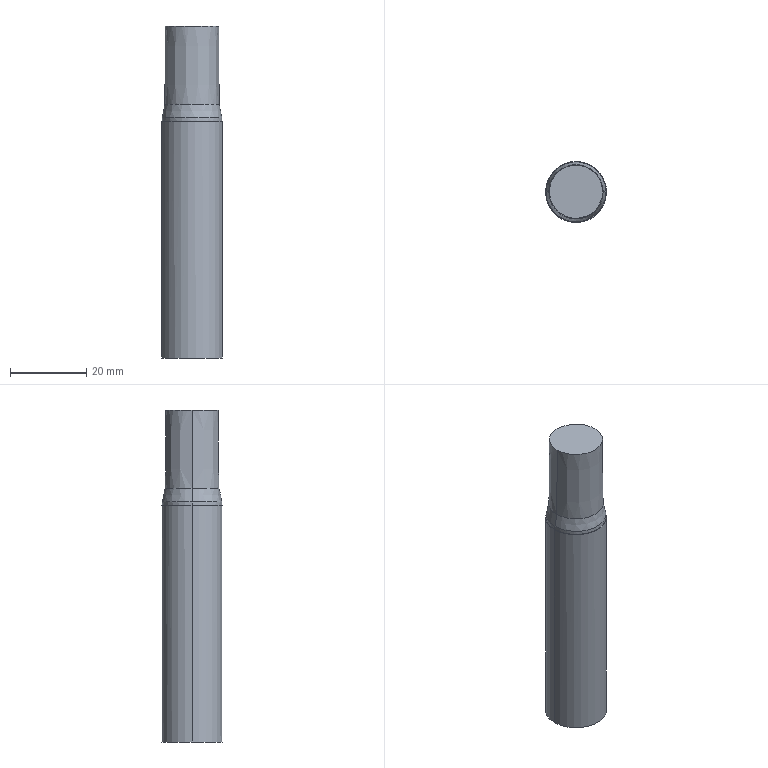Part | Creo | 1 solid | 11 faces | box 16 x 16 x 87.289 mm | volume 16530 mm3 | cylinder 4 | cone 4 | plane 3 | commonest cylinder face diameters 15.678 x2 16 x2
STEP:
#1=CARTESIAN_POINT('',(0.,0.,0.));
#2=DIRECTION('',(0.,0.,1.));
#3=DIRECTION('',(1.,0.,0.));
#4=AXIS2_PLACEMENT_3D('',#1,#2,#3);
#5=CARTESIAN_POINT('',(-166.942,-31.148,-153.441));
#6=VERTEX_POINT('',#5);
#7=CARTESIAN_POINT('',(-150.942,-31.148,-153.441));
#8=VERTEX_POINT('',#7);
#9=CARTESIAN_POINT('',(-158.942,-31.148,-153.441));
#10=DIRECTION('',(0.,0.,-1.));
#11=DIRECTION('',(-1.,0.,0.));
#12=AXIS2_PLACEMENT_3D('',#9,#10,#11);
#13=CIRCLE('',#12,8.);
#14=EDGE_CURVE('',#6,#8,#13,.T.);
#15=ORIENTED_EDGE('',*,*,#14,.T.);
#16=CARTESIAN_POINT('',(-150.942,-31.148,-91.317));
#17=VERTEX_POINT('',#16);
#18=CARTESIAN_POINT('',(-150.942,-31.148,-91.317));
#19=DIRECTION('',(0.,0.,-1.));
#20=VECTOR('',#19,62.125);
#21=LINE('',#18,#20);
#22=EDGE_CURVE('',#17,#8,#21,.T.);
#23=ORIENTED_EDGE('',*,*,#22,.F.);
#24=CARTESIAN_POINT('',(-166.942,-31.138,-91.296));
#25=VERTEX_POINT('',#24);
#26=CARTESIAN_POINT('',(-166.941,-30.196,-91.296));
#27=CARTESIAN_POINT('',(-166.597,-28.159,-91.296));
#28=CARTESIAN_POINT('',(-165.067,-25.793,-91.298));
#29=CARTESIAN_POINT('',(-163.339,-24.398,-91.301));
#30=CARTESIAN_POINT('',(-161.89,-23.654,-91.303));
#31=CARTESIAN_POINT('',(-160.637,-23.302,-91.304));
#32=CARTESIAN_POINT('',(-159.651,-23.169,-91.306));
#33=CARTESIAN_POINT('',(-158.937,-23.138,-91.306));
#34=CARTESIAN_POINT('',(-158.222,-23.17,-91.307));
#35=CARTESIAN_POINT('',(-157.236,-23.304,-91.309));
#36=CARTESIAN_POINT('',(-155.984,-23.658,-91.31));
#37=CARTESIAN_POINT('',(-154.536,-24.404,-91.312));
#38=CARTESIAN_POINT('',(-152.809,-25.801,-91.314));
#39=CARTESIAN_POINT('',(-151.283,-28.169,-91.316));
#40=CARTESIAN_POINT('',(-150.942,-30.206,-91.317));
#41=B_SPLINE_CURVE_WITH_KNOTS('',3,(#24,#26,#27,#28,#29,#30,#31,#32,#33,#34,#35,#36,#37,#38,#39,#40,#16),.UNSPECIFIED.,.F.,.F.,(4,1,1,1,1,1,1,1,1,1,1,1,1,1,4),(0.,0.125,0.25,0.3125,0.375,0.4375,0.4688,0.5,0.5312,0.5625,0.625,0.6875,0.75,0.875,1.),.UNSPECIFIED.);
#42=EDGE_CURVE('',#25,#17,#41,.T.);
#43=ORIENTED_EDGE('',*,*,#42,.F.);
#44=CARTESIAN_POINT('',(-166.942,-31.148,-91.296));
#45=VERTEX_POINT('',#44);
#46=CARTESIAN_POINT('',(-166.942,-31.145,-91.296));
#47=CARTESIAN_POINT('',(-166.942,-31.141,-91.296));
#48=CARTESIAN_POINT('',(-166.942,-31.138,-91.296));
#49=B_SPLINE_CURVE_WITH_KNOTS('',3,(#44,#46,#47,#48),.UNSPECIFIED.,.F.,.F.,(4,4),(0.,1.),.UNSPECIFIED.);
#50=EDGE_CURVE('',#45,#25,#49,.T.);
#51=ORIENTED_EDGE('',*,*,#50,.F.);
#52=CARTESIAN_POINT('',(-166.942,-31.148,-91.296));
#53=DIRECTION('',(-0.000000074,0.,-1.));
#54=VECTOR('',#53,62.146);
#55=LINE('',#52,#54);
#56=EDGE_CURVE('',#45,#6,#55,.T.);
#57=ORIENTED_EDGE('',*,*,#56,.T.);
#58=EDGE_LOOP('',(#15,#23,#43,#51,#57));
#59=FACE_OUTER_BOUND('',#58,.F.);
#60=CARTESIAN_POINT('',(-158.942,-31.148,508.193));
#61=DIRECTION('',(0.,0.,-1.));
#62=DIRECTION('',(-1.,0.,0.));
#63=AXIS2_PLACEMENT_3D('',#60,#61,#62);
#64=CYLINDRICAL_SURFACE('',#63,8.);
#65=ADVANCED_FACE('',(#59),#64,.T.);
#66=ORIENTED_EDGE('',*,*,#14,.F.);
#67=CARTESIAN_POINT('',(-158.942,-31.148,-153.441));
#68=DIRECTION('',(0.,0.,-1.));
#69=DIRECTION('',(1.,0.,0.));
#70=AXIS2_PLACEMENT_3D('',#67,#68,#69);
#71=CIRCLE('',#70,8.);
#72=EDGE_CURVE('',#8,#6,#71,.T.);
#73=ORIENTED_EDGE('',*,*,#72,.F.);
#74=EDGE_LOOP('',(#66,#73));
#75=FACE_OUTER_BOUND('',#74,.F.);
#76=CARTESIAN_POINT('',(5.725,319.968,-153.441));
#77=DIRECTION('',(0.,0.,-1.));
#78=DIRECTION('',(-1.,0.,0.));
#79=AXIS2_PLACEMENT_3D('',#76,#77,#78);
#80=PLANE('',#79);
#81=ADVANCED_FACE('',(#75),#80,.T.);
#82=ORIENTED_EDGE('',*,*,#72,.T.);
#83=ORIENTED_EDGE('',*,*,#56,.F.);
#84=CARTESIAN_POINT('',(-150.942,-31.158,-91.317));
#85=VERTEX_POINT('',#84);
#86=CARTESIAN_POINT('',(-150.942,-31.654,-91.317));
#87=CARTESIAN_POINT('',(-151.034,-32.628,-91.317));
#88=CARTESIAN_POINT('',(-151.44,-34.058,-91.316));
#89=CARTESIAN_POINT('',(-152.105,-35.389,-91.315));
#90=CARTESIAN_POINT('',(-152.991,-36.563,-91.314));
#91=CARTESIAN_POINT('',(-154.092,-37.569,-91.313));
#92=CARTESIAN_POINT('',(-155.36,-38.353,-91.311));
#93=CARTESIAN_POINT('',(-156.748,-38.889,-91.309));
#94=CARTESIAN_POINT('',(-158.208,-39.16,-91.307));
#95=CARTESIAN_POINT('',(-159.691,-39.159,-91.305));
#96=CARTESIAN_POINT('',(-161.146,-38.886,-91.304));
#97=CARTESIAN_POINT('',(-162.527,-38.35,-91.302));
#98=CARTESIAN_POINT('',(-163.788,-37.571,-91.3));
#99=CARTESIAN_POINT('',(-164.887,-36.569,-91.299));
#100=CARTESIAN_POINT('',(-165.774,-35.396,-91.297));
#101=CARTESIAN_POINT('',(-166.442,-34.063,-91.297));
#102=CARTESIAN_POINT('',(-166.85,-32.626,-91.296));
#103=CARTESIAN_POINT('',(-166.942,-31.647,-91.296));
#104=CARTESIAN_POINT('',(-166.942,-31.148,-91.296));
#105=B_SPLINE_CURVE_WITH_KNOTS('',3,(#84,#86,#87,#88,#89,#90,#91,#92,#93,#94,#95,#96,#97,#98,#99,#100,#101,#102,#103,#104),.UNSPECIFIED.,.F.,.F.,(4,1,1,1,1,1,1,1,1,1,1,1,1,1,1,1,1,4),(0.,0.05882,0.1176,0.1765,0.2353,0.2941,0.3529,0.4118,0.4706,0.5294,0.5882,0.6471,0.7059,0.7647,0.8235,0.8824,0.9412,1.),.UNSPECIFIED.);
#106=EDGE_CURVE('',#85,#45,#105,.T.);
#107=ORIENTED_EDGE('',*,*,#106,.F.);
#108=CARTESIAN_POINT('',(-150.942,-31.148,-91.317));
#109=CARTESIAN_POINT('',(-150.942,-31.152,-91.317));
#110=CARTESIAN_POINT('',(-150.942,-31.155,-91.317));
#111=CARTESIAN_POINT('',(-150.942,-31.158,-91.317));
#112=B_SPLINE_CURVE_WITH_KNOTS('',3,(#108,#109,#110,#111),.UNSPECIFIED.,.F.,.F.,(4,4),(0.,1.),.UNSPECIFIED.);
#113=EDGE_CURVE('',#17,#85,#112,.T.);
#114=ORIENTED_EDGE('',*,*,#113,.F.);
#115=ORIENTED_EDGE('',*,*,#22,.T.);
#116=EDGE_LOOP('',(#82,#83,#107,#114,#115));
#117=FACE_OUTER_BOUND('',#116,.F.);
#118=CARTESIAN_POINT('',(-158.942,-31.148,508.193));
#119=DIRECTION('',(0.,0.,-1.));
#120=DIRECTION('',(-1.,0.,0.));
#121=AXIS2_PLACEMENT_3D('',#118,#119,#120);
#122=CYLINDRICAL_SURFACE('',#121,8.);
#123=ADVANCED_FACE('',(#117),#122,.T.);
#124=ORIENTED_EDGE('',*,*,#106,.T.);
#125=ORIENTED_EDGE('',*,*,#50,.T.);
#126=ORIENTED_EDGE('',*,*,#42,.T.);
#127=ORIENTED_EDGE('',*,*,#113,.T.);
#128=EDGE_LOOP('',(#124,#125,#126,#127));
#129=FACE_OUTER_BOUND('',#128,.F.);
#130=CARTESIAN_POINT('',(-151.103,-31.158,-91.317));
#131=VERTEX_POINT('',#130);
#132=CARTESIAN_POINT('',(-151.103,-31.148,-91.317));
#133=VERTEX_POINT('',#132);
#134=CARTESIAN_POINT('',(-151.103,-31.155,-91.317));
#135=CARTESIAN_POINT('',(-151.103,-31.152,-91.317));
#136=CARTESIAN_POINT('',(-151.103,-31.148,-91.317));
#137=B_SPLINE_CURVE_WITH_KNOTS('',3,(#130,#134,#135,#136),.UNSPECIFIED.,.F.,.F.,(4,4),(0.,1.),.UNSPECIFIED.);
#138=EDGE_CURVE('',#131,#133,#137,.T.);
#139=ORIENTED_EDGE('',*,*,#138,.T.);
#140=CARTESIAN_POINT('',(-166.781,-31.138,-91.296));
#141=VERTEX_POINT('',#140);
#142=CARTESIAN_POINT('',(-151.103,-30.662,-91.317));
#143=CARTESIAN_POINT('',(-151.191,-29.708,-91.317));
#144=CARTESIAN_POINT('',(-151.587,-28.306,-91.316));
#145=CARTESIAN_POINT('',(-152.238,-27.001,-91.315));
#146=CARTESIAN_POINT('',(-153.104,-25.85,-91.314));
#147=CARTESIAN_POINT('',(-154.181,-24.863,-91.313));
#148=CARTESIAN_POINT('',(-155.422,-24.093,-91.311));
#149=CARTESIAN_POINT('',(-156.782,-23.566,-91.309));
#150=CARTESIAN_POINT('',(-158.213,-23.298,-91.307));
#151=CARTESIAN_POINT('',(-159.665,-23.298,-91.305));
#152=CARTESIAN_POINT('',(-161.092,-23.564,-91.304));
#153=CARTESIAN_POINT('',(-162.446,-24.086,-91.302));
#154=CARTESIAN_POINT('',(-163.683,-24.849,-91.3));
#155=CARTESIAN_POINT('',(-164.76,-25.829,-91.299));
#156=CARTESIAN_POINT('',(-165.631,-26.977,-91.298));
#157=CARTESIAN_POINT('',(-166.287,-28.283,-91.297));
#158=CARTESIAN_POINT('',(-166.689,-29.69,-91.296));
#159=CARTESIAN_POINT('',(-166.78,-30.65,-91.296));
#160=CARTESIAN_POINT('',(-166.781,-31.138,-91.296));
#161=B_SPLINE_CURVE_WITH_KNOTS('',3,(#132,#142,#143,#144,#145,#146,#147,#148,#149,#150,#151,#152,#153,#154,#155,#156,#157,#158,#159,#160),.UNSPECIFIED.,.F.,.F.,(4,1,1,1,1,1,1,1,1,1,1,1,1,1,1,1,1,4),(0.,0.05882,0.1176,0.1765,0.2353,0.2941,0.3529,0.4118,0.4706,0.5294,0.5882,0.6471,0.7059,0.7647,0.8235,0.8824,0.9412,1.),.UNSPECIFIED.);
#162=EDGE_CURVE('',#133,#141,#161,.T.);
#163=ORIENTED_EDGE('',*,*,#162,.T.);
#164=CARTESIAN_POINT('',(-166.781,-31.148,-91.296));
#165=VERTEX_POINT('',#164);
#166=CARTESIAN_POINT('',(-166.781,-31.142,-91.296));
#167=CARTESIAN_POINT('',(-166.781,-31.145,-91.296));
#168=B_SPLINE_CURVE_WITH_KNOTS('',3,(#140,#166,#167,#164),.UNSPECIFIED.,.F.,.F.,(4,4),(0.,1.),.UNSPECIFIED.);
#169=EDGE_CURVE('',#141,#165,#168,.T.);
#170=ORIENTED_EDGE('',*,*,#169,.T.);
#171=CARTESIAN_POINT('',(-166.781,-31.148,-91.296));
#172=CARTESIAN_POINT('',(-166.781,-32.072,-91.296));
#173=CARTESIAN_POINT('',(-166.446,-34.068,-91.297));
#174=CARTESIAN_POINT('',(-164.951,-36.388,-91.299));
#175=CARTESIAN_POINT('',(-163.259,-37.757,-91.301));
#176=CARTESIAN_POINT('',(-161.84,-38.488,-91.303));
#177=CARTESIAN_POINT('',(-160.613,-38.835,-91.304));
#178=CARTESIAN_POINT('',(-159.647,-38.966,-91.306));
#179=CARTESIAN_POINT('',(-158.947,-38.997,-91.306));
#180=CARTESIAN_POINT('',(-158.247,-38.967,-91.307));
#181=CARTESIAN_POINT('',(-157.28,-38.837,-91.309));
#182=CARTESIAN_POINT('',(-156.053,-38.491,-91.31));
#183=CARTESIAN_POINT('',(-154.633,-37.763,-91.312));
#184=CARTESIAN_POINT('',(-152.94,-36.395,-91.314));
#185=CARTESIAN_POINT('',(-151.441,-34.077,-91.316));
#186=CARTESIAN_POINT('',(-151.104,-32.082,-91.317));
#187=CARTESIAN_POINT('',(-151.103,-31.158,-91.317));
#188=B_SPLINE_CURVE_WITH_KNOTS('',3,(#171,#172,#173,#174,#175,#176,#177,#178,#179,#180,#181,#182,#183,#184,#185,#186,#187),.UNSPECIFIED.,.F.,.F.,(4,1,1,1,1,1,1,1,1,1,1,1,1,1,4),(0.,0.125,0.25,0.3125,0.375,0.4375,0.4688,0.5,0.5312,0.5625,0.625,0.6875,0.75,0.875,1.),.UNSPECIFIED.);
#189=EDGE_CURVE('',#165,#131,#188,.T.);
#190=ORIENTED_EDGE('',*,*,#189,.T.);
#191=EDGE_LOOP('',(#139,#163,#170,#190));
#192=FACE_BOUND('',#191,.F.);
#193=CARTESIAN_POINT('',(248.993,54.022,-91.842));
#194=DIRECTION('',(-0.001312,0.000001665,-1.));
#195=DIRECTION('',(-1.,0.,0.001312));
#196=AXIS2_PLACEMENT_3D('',#193,#194,#195);
#197=PLANE('',#196);
#198=ADVANCED_FACE('',(#129,#192),#197,.F.);
#199=CARTESIAN_POINT('',(-166.782,-31.148,-90.301));
#200=VERTEX_POINT('',#199);
#201=CARTESIAN_POINT('',(-151.102,-31.148,-90.301));
#202=VERTEX_POINT('',#201);
#203=CARTESIAN_POINT('',(-158.943,-31.148,-90.301));
#204=DIRECTION('',(0.00002709,0.,1.));
#205=DIRECTION('',(-1.,0.,0.00002709));
#206=AXIS2_PLACEMENT_3D('',#203,#204,#205);
#207=CIRCLE('',#206,7.841);
#208=EDGE_CURVE('',#200,#202,#207,.T.);
#209=ORIENTED_EDGE('',*,*,#208,.T.);
#210=CARTESIAN_POINT('',(-151.103,-31.148,-91.317));
#211=DIRECTION('',(0.0003927,0.000000008,1.));
#212=VECTOR('',#211,1.015);
#213=LINE('',#210,#212);
#214=EDGE_CURVE('',#133,#202,#213,.T.);
#215=ORIENTED_EDGE('',*,*,#214,.F.);
#216=ORIENTED_EDGE('',*,*,#138,.F.);
#217=ORIENTED_EDGE('',*,*,#189,.F.);
#218=CARTESIAN_POINT('',(-166.781,-31.148,-91.296));
#219=DIRECTION('',(-0.001462,0.,1.));
#220=VECTOR('',#219,0.995);
#221=LINE('',#218,#220);
#222=EDGE_CURVE('',#165,#200,#221,.T.);
#223=ORIENTED_EDGE('',*,*,#222,.T.);
#224=EDGE_LOOP('',(#209,#215,#216,#217,#223));
#225=FACE_OUTER_BOUND('',#224,.F.);
#226=CARTESIAN_POINT('',(-158.942,-31.148,-91.306));
#227=DIRECTION('',(0.,0.,1.));
#228=DIRECTION('',(1.,0.,0.));
#229=AXIS2_PLACEMENT_3D('',#226,#227,#228);
#230=CYLINDRICAL_SURFACE('',#229,7.839);
#231=ADVANCED_FACE('',(#225),#230,.T.);
#232=CARTESIAN_POINT('',(-166.079,-31.148,-86.784));
#233=VERTEX_POINT('',#232);
#234=CARTESIAN_POINT('',(-151.806,-31.148,-86.784));
#235=VERTEX_POINT('',#234);
#236=CARTESIAN_POINT('',(-158.942,-31.148,-86.784));
#237=DIRECTION('',(0.,0.,1.));
#238=DIRECTION('',(-1.,0.,0.));
#239=AXIS2_PLACEMENT_3D('',#236,#237,#238);
#240=CIRCLE('',#239,7.136);
#241=EDGE_CURVE('',#233,#235,#240,.T.);
#242=ORIENTED_EDGE('',*,*,#241,.T.);
#243=CARTESIAN_POINT('',(-151.806,-31.148,-86.784));
#244=DIRECTION('',(0.1961,0.,-0.9806));
#245=VECTOR('',#244,3.587);
#246=LINE('',#243,#245);
#247=EDGE_CURVE('',#235,#202,#246,.T.);
#248=ORIENTED_EDGE('',*,*,#247,.T.);
#249=ORIENTED_EDGE('',*,*,#208,.F.);
#250=CARTESIAN_POINT('',(-166.079,-31.148,-86.784));
#251=DIRECTION('',(-0.1962,0.,-0.9806));
#252=VECTOR('',#251,3.587);
#253=LINE('',#250,#252);
#254=EDGE_CURVE('',#233,#200,#253,.T.);
#255=ORIENTED_EDGE('',*,*,#254,.F.);
#256=EDGE_LOOP('',(#242,#248,#249,#255));
#257=FACE_OUTER_BOUND('',#256,.F.);
#258=CARTESIAN_POINT('',(-158.943,-31.148,-88.542));
#259=DIRECTION('',(-0.00002709,0.,-1.));
#260=DIRECTION('',(1.,0.,-0.00002709));
#261=AXIS2_PLACEMENT_3D('',#258,#259,#260);
#262=CONICAL_SURFACE('',#261,7.489,11.313);
#263=ADVANCED_FACE('',(#257),#262,.T.);
#264=ORIENTED_EDGE('',*,*,#241,.F.);
#265=CARTESIAN_POINT('',(-165.934,-31.148,-66.216));
#266=VERTEX_POINT('',#265);
#267=CARTESIAN_POINT('',(-165.934,-31.148,-66.216));
#268=DIRECTION('',(-0.007043,0.,-1.));
#269=VECTOR('',#268,20.568);
#270=LINE('',#267,#269);
#271=EDGE_CURVE('',#266,#233,#270,.T.);
#272=ORIENTED_EDGE('',*,*,#271,.F.);
#273=CARTESIAN_POINT('',(-159.821,-38.084,-66.153));
#274=VERTEX_POINT('',#273);
#275=CARTESIAN_POINT('',(-165.934,-31.148,-66.216));
#276=CARTESIAN_POINT('',(-165.934,-31.526,-66.212));
#277=CARTESIAN_POINT('',(-165.873,-32.271,-66.205));
#278=CARTESIAN_POINT('',(-165.604,-33.367,-66.194));
#279=CARTESIAN_POINT('',(-165.164,-34.402,-66.184));
#280=CARTESIAN_POINT('',(-164.565,-35.354,-66.175));
#281=CARTESIAN_POINT('',(-163.821,-36.197,-66.167));
#282=CARTESIAN_POINT('',(-162.952,-36.912,-66.161));
#283=CARTESIAN_POINT('',(-161.98,-37.478,-66.156));
#284=CARTESIAN_POINT('',(-160.927,-37.883,-66.153));
#285=CARTESIAN_POINT('',(-160.196,-38.037,-66.153));
#286=B_SPLINE_CURVE_WITH_KNOTS('',3,(#275,#276,#277,#278,#279,#280,#281,#282,#283,#284,#285,#273),.UNSPECIFIED.,.F.,.F.,(4,1,1,1,1,1,1,1,1,4),(0.,0.1111,0.2222,0.3333,0.4444,0.5556,0.6667,0.7778,0.8889,1.),.UNSPECIFIED.);
#287=EDGE_CURVE('',#266,#274,#286,.T.);
#288=ORIENTED_EDGE('',*,*,#287,.T.);
#289=CARTESIAN_POINT('',(-151.95,-31.148,-66.235));
#290=VERTEX_POINT('',#289);
#291=CARTESIAN_POINT('',(-159.821,-38.084,-66.153));
#292=CARTESIAN_POINT('',(-159.379,-38.14,-66.153));
#293=CARTESIAN_POINT('',(-158.502,-38.167,-66.154));
#294=CARTESIAN_POINT('',(-157.191,-37.96,-66.158));
#295=CARTESIAN_POINT('',(-155.947,-37.511,-66.164));
#296=CARTESIAN_POINT('',(-154.808,-36.838,-66.172));
#297=CARTESIAN_POINT('',(-153.816,-35.964,-66.183));
#298=CARTESIAN_POINT('',(-153.005,-34.919,-66.194));
#299=CARTESIAN_POINT('',(-152.404,-33.742,-66.207));
#300=CARTESIAN_POINT('',(-152.033,-32.467,-66.221));
#301=CARTESIAN_POINT('',(-151.95,-31.594,-66.23));
#302=CARTESIAN_POINT('',(-151.95,-31.148,-66.235));
#303=B_SPLINE_CURVE_WITH_KNOTS('',3,(#291,#292,#293,#294,#295,#296,#297,#298,#299,#300,#301,#302),.UNSPECIFIED.,.F.,.F.,(4,1,1,1,1,1,1,1,1,4),(0.,0.1111,0.2222,0.3333,0.4444,0.5556,0.6667,0.7778,0.8889,1.),.UNSPECIFIED.);
#304=EDGE_CURVE('',#274,#290,#303,.T.);
#305=ORIENTED_EDGE('',*,*,#304,.T.);
#306=CARTESIAN_POINT('',(-151.95,-31.148,-66.235));
#307=DIRECTION('',(0.006996,0.,-1.));
#308=VECTOR('',#307,20.55);
#309=LINE('',#306,#308);
#310=EDGE_CURVE('',#290,#235,#309,.T.);
#311=ORIENTED_EDGE('',*,*,#310,.T.);
#312=EDGE_LOOP('',(#264,#272,#288,#305,#311));
#313=FACE_OUTER_BOUND('',#312,.F.);
#314=CARTESIAN_POINT('',(-158.942,-31.148,-76.468));
#315=DIRECTION('',(0.,0.,-1.));
#316=DIRECTION('',(1.,0.,0.));
#317=AXIS2_PLACEMENT_3D('',#314,#315,#316);
#318=CONICAL_SURFACE('',#317,7.063,0.4);
#319=ADVANCED_FACE('',(#313),#318,.T.);
#320=CARTESIAN_POINT('',(-158.942,-31.148,-86.784));
#321=DIRECTION('',(0.,0.,1.));
#322=DIRECTION('',(1.,0.,0.));
#323=AXIS2_PLACEMENT_3D('',#320,#321,#322);
#324=CIRCLE('',#323,7.136);
#325=EDGE_CURVE('',#235,#233,#324,.T.);
#326=ORIENTED_EDGE('',*,*,#325,.F.);
#327=ORIENTED_EDGE('',*,*,#310,.F.);
#328=CARTESIAN_POINT('',(-151.95,-31.148,-66.235));
#329=CARTESIAN_POINT('',(-151.95,-30.685,-66.239));
#330=CARTESIAN_POINT('',(-152.04,-29.779,-66.249));
#331=CARTESIAN_POINT('',(-152.44,-28.453,-66.262));
#332=CARTESIAN_POINT('',(-153.094,-27.235,-66.273));
#333=CARTESIAN_POINT('',(-153.96,-26.178,-66.283));
#334=CARTESIAN_POINT('',(-155.03,-25.297,-66.291));
#335=CARTESIAN_POINT('',(-156.25,-24.646,-66.296));
#336=CARTESIAN_POINT('',(-157.572,-24.245,-66.298));
#337=CARTESIAN_POINT('',(-158.941,-24.111,-66.298));
#338=CARTESIAN_POINT('',(-160.309,-24.245,-66.295));
#339=CARTESIAN_POINT('',(-161.625,-24.643,-66.289));
#340=CARTESIAN_POINT('',(-162.84,-25.289,-66.281));
#341=CARTESIAN_POINT('',(-163.91,-26.164,-66.27));
#342=CARTESIAN_POINT('',(-164.78,-27.219,-66.258));
#343=CARTESIAN_POINT('',(-165.438,-28.44,-66.245));
#344=CARTESIAN_POINT('',(-165.843,-29.772,-66.231));
#345=CARTESIAN_POINT('',(-165.934,-30.683,-66.221));
#346=CARTESIAN_POINT('',(-165.934,-31.148,-66.216));
#347=B_SPLINE_CURVE_WITH_KNOTS('',3,(#328,#329,#330,#331,#332,#333,#334,#335,#336,#337,#338,#339,#340,#341,#342,#343,#344,#345,#346),.UNSPECIFIED.,.F.,.F.,(4,1,1,1,1,1,1,1,1,1,1,1,1,1,1,1,4),(0.,0.0625,0.125,0.1875,0.25,0.3125,0.375,0.4375,0.5,0.5625,0.625,0.6875,0.75,0.8125,0.875,0.9375,1.),.UNSPECIFIED.);
#348=EDGE_CURVE('',#290,#266,#347,.T.);
#349=ORIENTED_EDGE('',*,*,#348,.T.);
#350=ORIENTED_EDGE('',*,*,#271,.T.);
#351=EDGE_LOOP('',(#326,#327,#349,#350));
#352=FACE_OUTER_BOUND('',#351,.F.);
#353=CARTESIAN_POINT('',(-158.942,-31.148,-76.5));
#354=DIRECTION('',(0.,0.,-1.));
#355=DIRECTION('',(1.,0.,0.));
#356=AXIS2_PLACEMENT_3D('',#353,#354,#355);
#357=CONICAL_SURFACE('',#356,7.064,0.4);
#358=ADVANCED_FACE('',(#352),#357,.T.);
#359=ORIENTED_EDGE('',*,*,#325,.T.);
#360=ORIENTED_EDGE('',*,*,#254,.T.);
#361=CARTESIAN_POINT('',(-158.943,-31.148,-90.301));
#362=DIRECTION('',(0.00002709,0.,1.));
#363=DIRECTION('',(1.,0.,-0.00002709));
#364=AXIS2_PLACEMENT_3D('',#361,#362,#363);
#365=CIRCLE('',#364,7.841);
#366=EDGE_CURVE('',#202,#200,#365,.T.);
#367=ORIENTED_EDGE('',*,*,#366,.F.);
#368=ORIENTED_EDGE('',*,*,#247,.F.);
#369=EDGE_LOOP('',(#359,#360,#367,#368));
#370=FACE_OUTER_BOUND('',#369,.F.);
#371=CARTESIAN_POINT('',(-158.943,-31.148,-88.542));
#372=DIRECTION('',(-0.00002709,0.,-1.));
#373=DIRECTION('',(1.,0.,-0.00002709));
#374=AXIS2_PLACEMENT_3D('',#371,#372,#373);
#375=CONICAL_SURFACE('',#374,7.489,11.313);
#376=ADVANCED_FACE('',(#370),#375,.T.);
#377=ORIENTED_EDGE('',*,*,#366,.T.);
#378=ORIENTED_EDGE('',*,*,#222,.F.);
#379=ORIENTED_EDGE('',*,*,#169,.F.);
#380=ORIENTED_EDGE('',*,*,#162,.F.);
#381=ORIENTED_EDGE('',*,*,#214,.T.);
#382=EDGE_LOOP('',(#377,#378,#379,#380,#381));
#383=FACE_OUTER_BOUND('',#382,.F.);
#384=CARTESIAN_POINT('',(-158.942,-31.148,-91.306));
#385=DIRECTION('',(0.,0.,1.));
#386=DIRECTION('',(1.,0.,0.));
#387=AXIS2_PLACEMENT_3D('',#384,#385,#386);
#388=CYLINDRICAL_SURFACE('',#387,7.839);
#389=ADVANCED_FACE('',(#383),#388,.T.);
#390=ORIENTED_EDGE('',*,*,#304,.F.);
#391=ORIENTED_EDGE('',*,*,#287,.F.);
#392=ORIENTED_EDGE('',*,*,#348,.F.);
#393=EDGE_LOOP('',(#390,#391,#392));
#394=FACE_OUTER_BOUND('',#393,.F.);
#395=CARTESIAN_POINT('',(-158.942,-31.15,-66.225));
#396=DIRECTION('',(0.001305,0.0103,0.9999));
#397=DIRECTION('',(0.,0.9999,-0.0103));
#398=AXIS2_PLACEMENT_3D('',#395,#396,#397);
#399=PLANE('',#398);
#400=ADVANCED_FACE('',(#394),#399,.T.);
#401=CLOSED_SHELL('',(#65,#81,#123,#198,#231,#263,#319,#358,#376,#389,#400));
#402=MANIFOLD_SOLID_BREP('',#401);
#403=(LENGTH_UNIT()NAMED_UNIT(*)SI_UNIT(.MILLI.,.METRE.));
#404=UNCERTAINTY_MEASURE_WITH_UNIT(LENGTH_MEASURE(0.009018),#403,'','');
#405=(NAMED_UNIT(*)PLANE_ANGLE_UNIT()SI_UNIT($,.RADIAN.));
#406=PLANE_ANGLE_MEASURE_WITH_UNIT(PLANE_ANGLE_MEASURE(0.01745),#405);
#407=(CONVERSION_BASED_UNIT('DEGREE',#406)NAMED_UNIT(*)PLANE_ANGLE_UNIT());
#408=(NAMED_UNIT(*)SI_UNIT($,.STERADIAN.)SOLID_ANGLE_UNIT());
#409=(GEOMETRIC_REPRESENTATION_CONTEXT(3)GLOBAL_UNCERTAINTY_ASSIGNED_CONTEXT((#404))GLOBAL_UNIT_ASSIGNED_CONTEXT((#403,#407,#408))REPRESENTATION_CONTEXT('',''));
#410=ADVANCED_BREP_SHAPE_REPRESENTATION('',(#4,#402),#409);